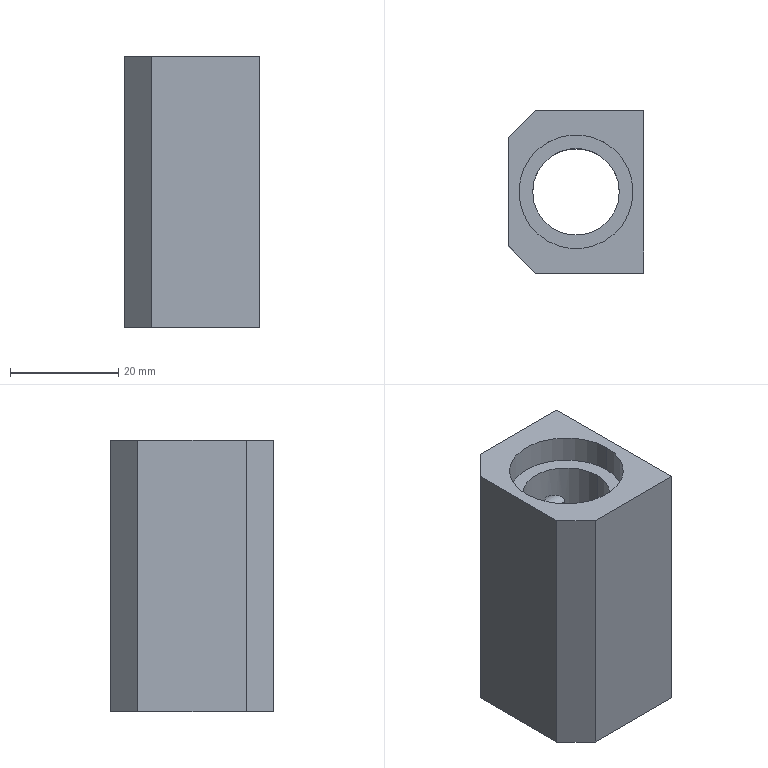Part | STEP file | MT-COMBO-119-S033 | 1 solid | 28 faces | box 25 x 30 x 50 mm | volume 24424 mm3 | cylinder 14 | plane 10 | cone 4 | commonest cylinder face diameters 3.3 x8 21 x4 16 x2
STEP:
#1=CARTESIAN_POINT('',(2.784,-7.5,14.15));
#2=VERTEX_POINT('',#1);
#3=CARTESIAN_POINT('',(2.784,-7.5,10.85));
#4=VERTEX_POINT('',#3);
#5=CARTESIAN_POINT('',(2.784,-7.5,14.15));
#6=CARTESIAN_POINT('',(3.09,-7.386,14.15));
#7=CARTESIAN_POINT('',(3.389,-7.254,14.139));
#8=CARTESIAN_POINT('',(3.967,-6.955,14.065));
#9=CARTESIAN_POINT('',(4.246,-6.787,14.002));
#10=CARTESIAN_POINT('',(4.631,-6.525,13.835));
#11=CARTESIAN_POINT('',(4.753,-6.437,13.767));
#12=CARTESIAN_POINT('',(4.976,-6.266,13.601));
#13=CARTESIAN_POINT('',(5.08,-6.181,13.501));
#14=CARTESIAN_POINT('',(5.256,-6.032,13.266));
#15=CARTESIAN_POINT('',(5.329,-5.967,13.129));
#16=CARTESIAN_POINT('',(5.404,-5.899,12.905));
#17=CARTESIAN_POINT('',(5.424,-5.881,12.828));
#18=CARTESIAN_POINT('',(5.45,-5.856,12.667));
#19=CARTESIAN_POINT('',(5.457,-5.85,12.583));
#20=CARTESIAN_POINT('',(5.457,-5.85,12.337));
#21=CARTESIAN_POINT('',(5.43,-5.875,12.172));
#22=CARTESIAN_POINT('',(5.33,-5.967,11.871));
#23=CARTESIAN_POINT('',(5.257,-6.032,11.734));
#24=CARTESIAN_POINT('',(4.99,-6.257,11.379));
#25=CARTESIAN_POINT('',(4.756,-6.44,11.219));
#26=CARTESIAN_POINT('',(4.246,-6.787,10.998));
#27=CARTESIAN_POINT('',(3.966,-6.955,10.935));
#28=CARTESIAN_POINT('',(3.388,-7.254,10.861));
#29=CARTESIAN_POINT('',(3.09,-7.386,10.85));
#30=CARTESIAN_POINT('',(2.784,-7.5,10.85));
#31=B_SPLINE_CURVE_WITH_KNOTS('',3,(#5,#6,#7,#8,#9,#10,#11,#12,#13,#14,#15,#16,#17,#18,#19,#20,#21,#22,#23,#24,#25,#26,#27,#28,#29,#30),.UNSPECIFIED.,.F.,.F.,(4,2,2,2,2,2,2,2,2,2,2,2,4),(0.0004038,0.001382,0.002361,0.00285,0.003339,0.003829,0.004073,0.004318,0.004807,0.005296,0.006275,0.007253,0.008232),.UNSPECIFIED.);
#32=EDGE_CURVE('',#2,#4,#31,.T.);
#33=ORIENTED_EDGE('',*,*,#32,.T.);
#34=CARTESIAN_POINT('',(12.5,-7.5,10.85));
#35=VERTEX_POINT('',#34);
#36=CARTESIAN_POINT('',(12.5,-7.5,10.85));
#37=DIRECTION('',(1.,0.,0.));
#38=VECTOR('',#37,1000.);
#39=LINE('',#36,#38);
#40=EDGE_CURVE('',#4,#35,#39,.T.);
#41=ORIENTED_EDGE('',*,*,#40,.T.);
#42=CARTESIAN_POINT('',(12.5,-7.5,14.15));
#43=VERTEX_POINT('',#42);
#44=CARTESIAN_POINT('',(12.5,-7.5,12.5));
#45=DIRECTION('',(-1.,0.,0.));
#46=DIRECTION('',(0.,0.,1.));
#47=AXIS2_PLACEMENT_3D('',#44,#45,#46);
#48=CIRCLE('',#47,1.65);
#49=EDGE_CURVE('',#43,#35,#48,.T.);
#50=ORIENTED_EDGE('',*,*,#49,.F.);
#51=CARTESIAN_POINT('',(12.5,-7.5,14.15));
#52=DIRECTION('',(1.,0.,0.));
#53=VECTOR('',#52,1000.);
#54=LINE('',#51,#53);
#55=EDGE_CURVE('',#2,#43,#54,.T.);
#56=ORIENTED_EDGE('',*,*,#55,.F.);
#57=EDGE_LOOP('',(#33,#41,#50,#56));
#58=FACE_OUTER_BOUND('',#57,.T.);
#59=CARTESIAN_POINT('',(12.5,-7.5,12.5));
#60=DIRECTION('',(1.,0.,0.));
#61=DIRECTION('',(0.,0.,1.));
#62=AXIS2_PLACEMENT_3D('',#59,#60,#61);
#63=CYLINDRICAL_SURFACE('',#62,1.65);
#64=ADVANCED_FACE('',(#58),#63,.F.);
#65=CARTESIAN_POINT('',(2.4,7.632,10.855));
#66=VERTEX_POINT('',#65);
#67=CARTESIAN_POINT('',(2.784,7.5,10.85));
#68=VERTEX_POINT('',#67);
#69=CARTESIAN_POINT('',(2.4,7.632,10.855));
#70=CARTESIAN_POINT('',(2.529,7.591,10.852));
#71=CARTESIAN_POINT('',(2.657,7.547,10.85));
#72=CARTESIAN_POINT('',(2.784,7.5,10.85));
#73=B_SPLINE_CURVE_WITH_KNOTS('',3,(#69,#70,#71,#72),.UNSPECIFIED.,.F.,.F.,(4,4),(0.,0.0004038),.UNSPECIFIED.);
#74=EDGE_CURVE('',#66,#68,#73,.T.);
#75=ORIENTED_EDGE('',*,*,#74,.T.);
#76=CARTESIAN_POINT('',(12.5,7.5,10.85));
#77=VERTEX_POINT('',#76);
#78=CARTESIAN_POINT('',(12.5,7.5,10.85));
#79=DIRECTION('',(1.,0.,0.));
#80=VECTOR('',#79,1000.);
#81=LINE('',#78,#80);
#82=EDGE_CURVE('',#68,#77,#81,.T.);
#83=ORIENTED_EDGE('',*,*,#82,.T.);
#84=CARTESIAN_POINT('',(12.5,7.5,14.15));
#85=VERTEX_POINT('',#84);
#86=CARTESIAN_POINT('',(12.5,7.5,12.5));
#87=DIRECTION('',(-1.,0.,0.));
#88=DIRECTION('',(0.,0.,1.));
#89=AXIS2_PLACEMENT_3D('',#86,#87,#88);
#90=CIRCLE('',#89,1.65);
#91=EDGE_CURVE('',#85,#77,#90,.T.);
#92=ORIENTED_EDGE('',*,*,#91,.F.);
#93=CARTESIAN_POINT('',(2.784,7.5,14.15));
#94=VERTEX_POINT('',#93);
#95=CARTESIAN_POINT('',(12.5,7.5,14.15));
#96=DIRECTION('',(1.,0.,0.));
#97=VECTOR('',#96,1000.);
#98=LINE('',#95,#97);
#99=EDGE_CURVE('',#94,#85,#98,.T.);
#100=ORIENTED_EDGE('',*,*,#99,.F.);
#101=CARTESIAN_POINT('',(2.4,7.632,14.145));
#102=VERTEX_POINT('',#101);
#103=CARTESIAN_POINT('',(2.784,7.5,14.15));
#104=CARTESIAN_POINT('',(2.657,7.547,14.15));
#105=CARTESIAN_POINT('',(2.529,7.591,14.148));
#106=CARTESIAN_POINT('',(2.4,7.632,14.145));
#107=B_SPLINE_CURVE_WITH_KNOTS('',3,(#103,#104,#105,#106),.UNSPECIFIED.,.F.,.F.,(4,4),(0.008232,0.008636),.UNSPECIFIED.);
#108=EDGE_CURVE('',#94,#102,#107,.T.);
#109=ORIENTED_EDGE('',*,*,#108,.T.);
#110=CARTESIAN_POINT('',(2.4,7.5,12.5));
#111=DIRECTION('',(-1.,0.,0.));
#112=DIRECTION('',(0.,0.,1.));
#113=AXIS2_PLACEMENT_3D('',#110,#111,#112);
#114=CIRCLE('',#113,1.65);
#115=EDGE_CURVE('',#102,#66,#114,.T.);
#116=ORIENTED_EDGE('',*,*,#115,.T.);
#117=EDGE_LOOP('',(#75,#83,#92,#100,#109,#116));
#118=FACE_OUTER_BOUND('',#117,.T.);
#119=CARTESIAN_POINT('',(12.5,7.5,12.5));
#120=DIRECTION('',(1.,0.,0.));
#121=DIRECTION('',(0.,0.,1.));
#122=AXIS2_PLACEMENT_3D('',#119,#120,#121);
#123=CYLINDRICAL_SURFACE('',#122,1.65);
#124=ADVANCED_FACE('',(#118),#123,.F.);
#125=CARTESIAN_POINT('',(2.4,7.632,-14.145));
#126=VERTEX_POINT('',#125);
#127=CARTESIAN_POINT('',(2.784,7.5,-14.15));
#128=VERTEX_POINT('',#127);
#129=CARTESIAN_POINT('',(2.4,7.632,-14.145));
#130=CARTESIAN_POINT('',(2.529,7.591,-14.148));
#131=CARTESIAN_POINT('',(2.657,7.547,-14.15));
#132=CARTESIAN_POINT('',(2.784,7.5,-14.15));
#133=B_SPLINE_CURVE_WITH_KNOTS('',3,(#129,#130,#131,#132),.UNSPECIFIED.,.F.,.F.,(4,4),(0.,0.0004038),.UNSPECIFIED.);
#134=EDGE_CURVE('',#126,#128,#133,.T.);
#135=ORIENTED_EDGE('',*,*,#134,.T.);
#136=CARTESIAN_POINT('',(12.5,7.5,-14.15));
#137=VERTEX_POINT('',#136);
#138=CARTESIAN_POINT('',(12.5,7.5,-14.15));
#139=DIRECTION('',(1.,0.,0.));
#140=VECTOR('',#139,1000.);
#141=LINE('',#138,#140);
#142=EDGE_CURVE('',#128,#137,#141,.T.);
#143=ORIENTED_EDGE('',*,*,#142,.T.);
#144=CARTESIAN_POINT('',(12.5,7.5,-10.85));
#145=VERTEX_POINT('',#144);
#146=CARTESIAN_POINT('',(12.5,7.5,-12.5));
#147=DIRECTION('',(-1.,0.,0.));
#148=DIRECTION('',(0.,0.,1.));
#149=AXIS2_PLACEMENT_3D('',#146,#147,#148);
#150=CIRCLE('',#149,1.65);
#151=EDGE_CURVE('',#145,#137,#150,.T.);
#152=ORIENTED_EDGE('',*,*,#151,.F.);
#153=CARTESIAN_POINT('',(2.784,7.5,-10.85));
#154=VERTEX_POINT('',#153);
#155=CARTESIAN_POINT('',(12.5,7.5,-10.85));
#156=DIRECTION('',(1.,0.,0.));
#157=VECTOR('',#156,1000.);
#158=LINE('',#155,#157);
#159=EDGE_CURVE('',#154,#145,#158,.T.);
#160=ORIENTED_EDGE('',*,*,#159,.F.);
#161=CARTESIAN_POINT('',(2.4,7.632,-10.855));
#162=VERTEX_POINT('',#161);
#163=CARTESIAN_POINT('',(2.784,7.5,-10.85));
#164=CARTESIAN_POINT('',(2.657,7.547,-10.85));
#165=CARTESIAN_POINT('',(2.529,7.591,-10.852));
#166=CARTESIAN_POINT('',(2.4,7.632,-10.855));
#167=B_SPLINE_CURVE_WITH_KNOTS('',3,(#163,#164,#165,#166),.UNSPECIFIED.,.F.,.F.,(4,4),(0.008232,0.008636),.UNSPECIFIED.);
#168=EDGE_CURVE('',#154,#162,#167,.T.);
#169=ORIENTED_EDGE('',*,*,#168,.T.);
#170=CARTESIAN_POINT('',(2.4,7.5,-12.5));
#171=DIRECTION('',(-1.,0.,0.));
#172=DIRECTION('',(0.,0.,1.));
#173=AXIS2_PLACEMENT_3D('',#170,#171,#172);
#174=CIRCLE('',#173,1.65);
#175=EDGE_CURVE('',#162,#126,#174,.T.);
#176=ORIENTED_EDGE('',*,*,#175,.T.);
#177=EDGE_LOOP('',(#135,#143,#152,#160,#169,#176));
#178=FACE_OUTER_BOUND('',#177,.T.);
#179=CARTESIAN_POINT('',(12.5,7.5,-12.5));
#180=DIRECTION('',(1.,0.,0.));
#181=DIRECTION('',(0.,0.,1.));
#182=AXIS2_PLACEMENT_3D('',#179,#180,#181);
#183=CYLINDRICAL_SURFACE('',#182,1.65);
#184=ADVANCED_FACE('',(#178),#183,.F.);
#185=CARTESIAN_POINT('',(2.784,-7.5,-10.85));
#186=VERTEX_POINT('',#185);
#187=CARTESIAN_POINT('',(2.784,-7.5,-14.15));
#188=VERTEX_POINT('',#187);
#189=CARTESIAN_POINT('',(2.784,-7.5,-10.85));
#190=CARTESIAN_POINT('',(3.09,-7.386,-10.85));
#191=CARTESIAN_POINT('',(3.389,-7.254,-10.861));
#192=CARTESIAN_POINT('',(3.967,-6.955,-10.935));
#193=CARTESIAN_POINT('',(4.246,-6.787,-10.998));
#194=CARTESIAN_POINT('',(4.631,-6.525,-11.165));
#195=CARTESIAN_POINT('',(4.753,-6.437,-11.233));
#196=CARTESIAN_POINT('',(4.976,-6.266,-11.399));
#197=CARTESIAN_POINT('',(5.08,-6.181,-11.499));
#198=CARTESIAN_POINT('',(5.256,-6.032,-11.734));
#199=CARTESIAN_POINT('',(5.329,-5.967,-11.871));
#200=CARTESIAN_POINT('',(5.404,-5.899,-12.095));
#201=CARTESIAN_POINT('',(5.424,-5.881,-12.172));
#202=CARTESIAN_POINT('',(5.45,-5.856,-12.333));
#203=CARTESIAN_POINT('',(5.457,-5.85,-12.417));
#204=CARTESIAN_POINT('',(5.457,-5.85,-12.663));
#205=CARTESIAN_POINT('',(5.43,-5.875,-12.828));
#206=CARTESIAN_POINT('',(5.33,-5.967,-13.129));
#207=CARTESIAN_POINT('',(5.257,-6.032,-13.266));
#208=CARTESIAN_POINT('',(4.99,-6.257,-13.621));
#209=CARTESIAN_POINT('',(4.756,-6.44,-13.781));
#210=CARTESIAN_POINT('',(4.246,-6.787,-14.002));
#211=CARTESIAN_POINT('',(3.966,-6.955,-14.065));
#212=CARTESIAN_POINT('',(3.388,-7.254,-14.139));
#213=CARTESIAN_POINT('',(3.09,-7.386,-14.15));
#214=CARTESIAN_POINT('',(2.784,-7.5,-14.15));
#215=B_SPLINE_CURVE_WITH_KNOTS('',3,(#189,#190,#191,#192,#193,#194,#195,#196,#197,#198,#199,#200,#201,#202,#203,#204,#205,#206,#207,#208,#209,#210,#211,#212,#213,#214),.UNSPECIFIED.,.F.,.F.,(4,2,2,2,2,2,2,2,2,2,2,2,4),(0.0004038,0.001382,0.002361,0.00285,0.003339,0.003829,0.004073,0.004318,0.004807,0.005296,0.006275,0.007253,0.008232),.UNSPECIFIED.);
#216=EDGE_CURVE('',#186,#188,#215,.T.);
#217=ORIENTED_EDGE('',*,*,#216,.T.);
#218=CARTESIAN_POINT('',(12.5,-7.5,-14.15));
#219=VERTEX_POINT('',#218);
#220=CARTESIAN_POINT('',(12.5,-7.5,-14.15));
#221=DIRECTION('',(1.,0.,0.));
#222=VECTOR('',#221,1000.);
#223=LINE('',#220,#222);
#224=EDGE_CURVE('',#188,#219,#223,.T.);
#225=ORIENTED_EDGE('',*,*,#224,.T.);
#226=CARTESIAN_POINT('',(12.5,-7.5,-10.85));
#227=VERTEX_POINT('',#226);
#228=CARTESIAN_POINT('',(12.5,-7.5,-12.5));
#229=DIRECTION('',(-1.,0.,0.));
#230=DIRECTION('',(0.,0.,1.));
#231=AXIS2_PLACEMENT_3D('',#228,#229,#230);
#232=CIRCLE('',#231,1.65);
#233=EDGE_CURVE('',#227,#219,#232,.T.);
#234=ORIENTED_EDGE('',*,*,#233,.F.);
#235=CARTESIAN_POINT('',(12.5,-7.5,-10.85));
#236=DIRECTION('',(1.,0.,0.));
#237=VECTOR('',#236,1000.);
#238=LINE('',#235,#237);
#239=EDGE_CURVE('',#186,#227,#238,.T.);
#240=ORIENTED_EDGE('',*,*,#239,.F.);
#241=EDGE_LOOP('',(#217,#225,#234,#240));
#242=FACE_OUTER_BOUND('',#241,.T.);
#243=CARTESIAN_POINT('',(12.5,-7.5,-12.5));
#244=DIRECTION('',(1.,0.,0.));
#245=DIRECTION('',(0.,0.,1.));
#246=AXIS2_PLACEMENT_3D('',#243,#244,#245);
#247=CYLINDRICAL_SURFACE('',#246,1.65);
#248=ADVANCED_FACE('',(#242),#247,.F.);
#249=CARTESIAN_POINT('',(-10.5,0.,-20.));
#250=VERTEX_POINT('',#249);
#251=CARTESIAN_POINT('',(10.5,0.,-20.));
#252=VERTEX_POINT('',#251);
#253=CARTESIAN_POINT('',(0.,0.,-20.));
#254=DIRECTION('',(0.,0.,-1.));
#255=DIRECTION('',(-1.,0.,0.));
#256=AXIS2_PLACEMENT_3D('',#253,#254,#255);
#257=CIRCLE('',#256,10.5);
#258=EDGE_CURVE('',#250,#252,#257,.T.);
#259=ORIENTED_EDGE('',*,*,#258,.F.);
#260=CARTESIAN_POINT('',(-10.5,0.,-25.));
#261=VERTEX_POINT('',#260);
#262=CARTESIAN_POINT('',(-10.5,0.,-20.));
#263=DIRECTION('',(0.,0.,-1.));
#264=VECTOR('',#263,1000.);
#265=LINE('',#262,#264);
#266=EDGE_CURVE('',#250,#261,#265,.T.);
#267=ORIENTED_EDGE('',*,*,#266,.T.);
#268=CARTESIAN_POINT('',(10.5,0.,-25.));
#269=VERTEX_POINT('',#268);
#270=CARTESIAN_POINT('',(0.,0.,-25.));
#271=DIRECTION('',(0.,0.,-1.));
#272=DIRECTION('',(-1.,0.,0.));
#273=AXIS2_PLACEMENT_3D('',#270,#271,#272);
#274=CIRCLE('',#273,10.5);
#275=EDGE_CURVE('',#261,#269,#274,.T.);
#276=ORIENTED_EDGE('',*,*,#275,.T.);
#277=CARTESIAN_POINT('',(10.5,0.,-20.));
#278=DIRECTION('',(0.,0.,-1.));
#279=VECTOR('',#278,1000.);
#280=LINE('',#277,#279);
#281=EDGE_CURVE('',#252,#269,#280,.T.);
#282=ORIENTED_EDGE('',*,*,#281,.F.);
#283=EDGE_LOOP('',(#259,#267,#276,#282));
#284=FACE_OUTER_BOUND('',#283,.T.);
#285=CARTESIAN_POINT('',(0.,0.,-20.));
#286=DIRECTION('',(0.,0.,-1.));
#287=DIRECTION('',(1.,0.,0.));
#288=AXIS2_PLACEMENT_3D('',#285,#286,#287);
#289=CYLINDRICAL_SURFACE('',#288,10.5);
#290=ADVANCED_FACE('',(#284),#289,.F.);
#291=CARTESIAN_POINT('',(-10.5,0.,20.));
#292=VERTEX_POINT('',#291);
#293=CARTESIAN_POINT('',(10.5,0.,20.));
#294=VERTEX_POINT('',#293);
#295=CARTESIAN_POINT('',(0.,0.,20.));
#296=DIRECTION('',(0.,0.,-1.));
#297=DIRECTION('',(-1.,0.,0.));
#298=AXIS2_PLACEMENT_3D('',#295,#296,#297);
#299=CIRCLE('',#298,10.5);
#300=EDGE_CURVE('',#292,#294,#299,.T.);
#301=ORIENTED_EDGE('',*,*,#300,.T.);
#302=CARTESIAN_POINT('',(10.5,0.,25.));
#303=VERTEX_POINT('',#302);
#304=CARTESIAN_POINT('',(10.5,0.,20.));
#305=DIRECTION('',(0.,0.,1.));
#306=VECTOR('',#305,1000.);
#307=LINE('',#304,#306);
#308=EDGE_CURVE('',#294,#303,#307,.T.);
#309=ORIENTED_EDGE('',*,*,#308,.T.);
#310=CARTESIAN_POINT('',(-10.5,0.,25.));
#311=VERTEX_POINT('',#310);
#312=CARTESIAN_POINT('',(0.,0.,25.));
#313=DIRECTION('',(0.,0.,-1.));
#314=DIRECTION('',(-1.,0.,0.));
#315=AXIS2_PLACEMENT_3D('',#312,#313,#314);
#316=CIRCLE('',#315,10.5);
#317=EDGE_CURVE('',#311,#303,#316,.T.);
#318=ORIENTED_EDGE('',*,*,#317,.F.);
#319=CARTESIAN_POINT('',(-10.5,0.,20.));
#320=DIRECTION('',(0.,0.,1.));
#321=VECTOR('',#320,1000.);
#322=LINE('',#319,#321);
#323=EDGE_CURVE('',#292,#311,#322,.T.);
#324=ORIENTED_EDGE('',*,*,#323,.F.);
#325=EDGE_LOOP('',(#301,#309,#318,#324));
#326=FACE_OUTER_BOUND('',#325,.T.);
#327=CARTESIAN_POINT('',(0.,0.,20.));
#328=DIRECTION('',(0.,0.,1.));
#329=DIRECTION('',(-1.,0.,0.));
#330=AXIS2_PLACEMENT_3D('',#327,#328,#329);
#331=CYLINDRICAL_SURFACE('',#330,10.5);
#332=ADVANCED_FACE('',(#326),#331,.F.);
#333=CARTESIAN_POINT('',(2.4,7.632,-10.855));
#334=CARTESIAN_POINT('',(2.244,7.68,-11.119));
#335=CARTESIAN_POINT('',(2.089,7.724,-11.384));
#336=CARTESIAN_POINT('',(1.867,7.78,-11.789));
#337=CARTESIAN_POINT('',(1.794,7.797,-11.924));
#338=CARTESIAN_POINT('',(1.698,7.818,-12.135));
#339=CARTESIAN_POINT('',(1.668,7.824,-12.207));
#340=CARTESIAN_POINT('',(1.624,7.834,-12.355));
#341=CARTESIAN_POINT('',(1.61,7.836,-12.432));
#342=CARTESIAN_POINT('',(1.612,7.836,-12.586));
#343=CARTESIAN_POINT('',(1.628,7.833,-12.663));
#344=CARTESIAN_POINT('',(1.675,7.823,-12.81));
#345=CARTESIAN_POINT('',(1.704,7.816,-12.88));
#346=CARTESIAN_POINT('',(1.8,7.795,-13.087));
#347=CARTESIAN_POINT('',(1.872,7.778,-13.222));
#348=CARTESIAN_POINT('',(2.093,7.723,-13.622));
#349=CARTESIAN_POINT('',(2.246,7.68,-13.884));
#350=CARTESIAN_POINT('',(2.4,7.632,-14.145));
#351=B_SPLINE_CURVE_WITH_KNOTS('',3,(#333,#334,#335,#336,#337,#338,#339,#340,#341,#342,#343,#344,#345,#346,#347,#348,#349,#350),.UNSPECIFIED.,.F.,.F.,(4,2,2,2,2,2,2,2,4),(0.0001976,0.001128,0.001593,0.001825,0.002058,0.00229,0.002523,0.002988,0.003918),.UNSPECIFIED.);
#352=EDGE_CURVE('',#162,#126,#351,.T.);
#353=ORIENTED_EDGE('',*,*,#352,.F.);
#354=ORIENTED_EDGE('',*,*,#168,.F.);
#355=CARTESIAN_POINT('',(2.784,7.5,-14.15));
#356=CARTESIAN_POINT('',(3.09,7.386,-14.15));
#357=CARTESIAN_POINT('',(3.389,7.254,-14.139));
#358=CARTESIAN_POINT('',(3.967,6.955,-14.065));
#359=CARTESIAN_POINT('',(4.246,6.787,-14.002));
#360=CARTESIAN_POINT('',(4.631,6.525,-13.835));
#361=CARTESIAN_POINT('',(4.753,6.437,-13.767));
#362=CARTESIAN_POINT('',(4.976,6.266,-13.601));
#363=CARTESIAN_POINT('',(5.08,6.181,-13.501));
#364=CARTESIAN_POINT('',(5.256,6.032,-13.266));
#365=CARTESIAN_POINT('',(5.329,5.967,-13.129));
#366=CARTESIAN_POINT('',(5.404,5.899,-12.905));
#367=CARTESIAN_POINT('',(5.424,5.881,-12.828));
#368=CARTESIAN_POINT('',(5.45,5.856,-12.667));
#369=CARTESIAN_POINT('',(5.457,5.85,-12.583));
#370=CARTESIAN_POINT('',(5.457,5.85,-12.337));
#371=CARTESIAN_POINT('',(5.43,5.875,-12.172));
#372=CARTESIAN_POINT('',(5.33,5.967,-11.871));
#373=CARTESIAN_POINT('',(5.257,6.032,-11.734));
#374=CARTESIAN_POINT('',(4.99,6.257,-11.379));
#375=CARTESIAN_POINT('',(4.756,6.44,-11.219));
#376=CARTESIAN_POINT('',(4.246,6.787,-10.998));
#377=CARTESIAN_POINT('',(3.966,6.955,-10.935));
#378=CARTESIAN_POINT('',(3.388,7.254,-10.861));
#379=CARTESIAN_POINT('',(3.09,7.386,-10.85));
#380=CARTESIAN_POINT('',(2.784,7.5,-10.85));
#381=B_SPLINE_CURVE_WITH_KNOTS('',3,(#355,#356,#357,#358,#359,#360,#361,#362,#363,#364,#365,#366,#367,#368,#369,#370,#371,#372,#373,#374,#375,#376,#377,#378,#379,#380),.UNSPECIFIED.,.F.,.F.,(4,2,2,2,2,2,2,2,2,2,2,2,4),(0.0004038,0.001382,0.002361,0.00285,0.003339,0.003829,0.004073,0.004318,0.004807,0.005296,0.006275,0.007253,0.008232),.UNSPECIFIED.);
#382=EDGE_CURVE('',#128,#154,#381,.T.);
#383=ORIENTED_EDGE('',*,*,#382,.F.);
#384=ORIENTED_EDGE('',*,*,#134,.F.);
#385=EDGE_LOOP('',(#353,#354,#383,#384));
#386=FACE_BOUND('',#385,.T.);
#387=CARTESIAN_POINT('',(2.4,7.632,14.145));
#388=CARTESIAN_POINT('',(2.244,7.68,13.881));
#389=CARTESIAN_POINT('',(2.089,7.724,13.616));
#390=CARTESIAN_POINT('',(1.867,7.78,13.211));
#391=CARTESIAN_POINT('',(1.794,7.797,13.076));
#392=CARTESIAN_POINT('',(1.698,7.818,12.865));
#393=CARTESIAN_POINT('',(1.668,7.824,12.793));
#394=CARTESIAN_POINT('',(1.624,7.834,12.645));
#395=CARTESIAN_POINT('',(1.61,7.836,12.568));
#396=CARTESIAN_POINT('',(1.612,7.836,12.414));
#397=CARTESIAN_POINT('',(1.628,7.833,12.337));
#398=CARTESIAN_POINT('',(1.675,7.823,12.19));
#399=CARTESIAN_POINT('',(1.704,7.816,12.12));
#400=CARTESIAN_POINT('',(1.8,7.795,11.913));
#401=CARTESIAN_POINT('',(1.872,7.778,11.778));
#402=CARTESIAN_POINT('',(2.093,7.723,11.378));
#403=CARTESIAN_POINT('',(2.246,7.68,11.116));
#404=CARTESIAN_POINT('',(2.4,7.632,10.855));
#405=B_SPLINE_CURVE_WITH_KNOTS('',3,(#387,#388,#389,#390,#391,#392,#393,#394,#395,#396,#397,#398,#399,#400,#401,#402,#403,#404),.UNSPECIFIED.,.F.,.F.,(4,2,2,2,2,2,2,2,4),(0.0001976,0.001128,0.001593,0.001825,0.002058,0.00229,0.002523,0.002988,0.003918),.UNSPECIFIED.);
#406=EDGE_CURVE('',#102,#66,#405,.T.);
#407=ORIENTED_EDGE('',*,*,#406,.F.);
#408=ORIENTED_EDGE('',*,*,#108,.F.);
#409=CARTESIAN_POINT('',(2.784,7.5,10.85));
#410=CARTESIAN_POINT('',(3.09,7.386,10.85));
#411=CARTESIAN_POINT('',(3.389,7.254,10.861));
#412=CARTESIAN_POINT('',(3.967,6.955,10.935));
#413=CARTESIAN_POINT('',(4.246,6.787,10.998));
#414=CARTESIAN_POINT('',(4.631,6.525,11.165));
#415=CARTESIAN_POINT('',(4.753,6.437,11.233));
#416=CARTESIAN_POINT('',(4.976,6.266,11.399));
#417=CARTESIAN_POINT('',(5.08,6.181,11.499));
#418=CARTESIAN_POINT('',(5.256,6.032,11.734));
#419=CARTESIAN_POINT('',(5.329,5.967,11.871));
#420=CARTESIAN_POINT('',(5.404,5.899,12.095));
#421=CARTESIAN_POINT('',(5.424,5.881,12.172));
#422=CARTESIAN_POINT('',(5.45,5.856,12.333));
#423=CARTESIAN_POINT('',(5.457,5.85,12.417));
#424=CARTESIAN_POINT('',(5.457,5.85,12.663));
#425=CARTESIAN_POINT('',(5.43,5.875,12.828));
#426=CARTESIAN_POINT('',(5.33,5.967,13.129));
#427=CARTESIAN_POINT('',(5.257,6.032,13.266));
#428=CARTESIAN_POINT('',(4.99,6.257,13.621));
#429=CARTESIAN_POINT('',(4.756,6.44,13.781));
#430=CARTESIAN_POINT('',(4.246,6.787,14.002));
#431=CARTESIAN_POINT('',(3.966,6.955,14.065));
#432=CARTESIAN_POINT('',(3.388,7.254,14.139));
#433=CARTESIAN_POINT('',(3.09,7.386,14.15));
#434=CARTESIAN_POINT('',(2.784,7.5,14.15));
#435=B_SPLINE_CURVE_WITH_KNOTS('',3,(#409,#410,#411,#412,#413,#414,#415,#416,#417,#418,#419,#420,#421,#422,#423,#424,#425,#426,#427,#428,#429,#430,#431,#432,#433,#434),.UNSPECIFIED.,.F.,.F.,(4,2,2,2,2,2,2,2,2,2,2,2,4),(0.0004038,0.001382,0.002361,0.00285,0.003339,0.003829,0.004073,0.004318,0.004807,0.005296,0.006275,0.007253,0.008232),.UNSPECIFIED.);
#436=EDGE_CURVE('',#68,#94,#435,.T.);
#437=ORIENTED_EDGE('',*,*,#436,.F.);
#438=ORIENTED_EDGE('',*,*,#74,.F.);
#439=EDGE_LOOP('',(#407,#408,#437,#438));
#440=FACE_BOUND('',#439,.T.);
#441=CARTESIAN_POINT('',(8.,0.,20.));
#442=VERTEX_POINT('',#441);
#443=CARTESIAN_POINT('',(-8.,0.,20.));
#444=VERTEX_POINT('',#443);
#445=CARTESIAN_POINT('',(0.,0.,20.));
#446=DIRECTION('',(0.,0.,1.));
#447=DIRECTION('',(-1.,0.,0.));
#448=AXIS2_PLACEMENT_3D('',#445,#446,#447);
#449=CIRCLE('',#448,8.);
#450=EDGE_CURVE('',#442,#444,#449,.T.);
#451=ORIENTED_EDGE('',*,*,#450,.T.);
#452=CARTESIAN_POINT('',(-8.,0.,-20.));
#453=VERTEX_POINT('',#452);
#454=CARTESIAN_POINT('',(-8.,0.,25.));
#455=DIRECTION('',(0.,0.,-1.));
#456=VECTOR('',#455,1000.);
#457=LINE('',#454,#456);
#458=EDGE_CURVE('',#444,#453,#457,.T.);
#459=ORIENTED_EDGE('',*,*,#458,.T.);
#460=CARTESIAN_POINT('',(8.,0.,-20.));
#461=VERTEX_POINT('',#460);
#462=CARTESIAN_POINT('',(0.,0.,-20.));
#463=DIRECTION('',(0.,0.,-1.));
#464=DIRECTION('',(1.,0.,0.));
#465=AXIS2_PLACEMENT_3D('',#462,#463,#464);
#466=CIRCLE('',#465,8.);
#467=EDGE_CURVE('',#453,#461,#466,.T.);
#468=ORIENTED_EDGE('',*,*,#467,.T.);
#469=CARTESIAN_POINT('',(8.,0.,25.));
#470=DIRECTION('',(0.,0.,-1.));
#471=VECTOR('',#470,1000.);
#472=LINE('',#469,#471);
#473=EDGE_CURVE('',#442,#461,#472,.T.);
#474=ORIENTED_EDGE('',*,*,#473,.F.);
#475=EDGE_LOOP('',(#451,#459,#468,#474));
#476=FACE_OUTER_BOUND('',#475,.T.);
#477=CARTESIAN_POINT('',(0.,0.,25.));
#478=DIRECTION('',(0.,0.,-1.));
#479=DIRECTION('',(1.,0.,0.));
#480=AXIS2_PLACEMENT_3D('',#477,#478,#479);
#481=CYLINDRICAL_SURFACE('',#480,8.);
#482=ADVANCED_FACE('',(#386,#440,#476),#481,.F.);
#483=ORIENTED_EDGE('',*,*,#458,.F.);
#484=CARTESIAN_POINT('',(0.,0.,20.));
#485=DIRECTION('',(0.,0.,1.));
#486=DIRECTION('',(-1.,0.,0.));
#487=AXIS2_PLACEMENT_3D('',#484,#485,#486);
#488=CIRCLE('',#487,8.);
#489=EDGE_CURVE('',#444,#442,#488,.T.);
#490=ORIENTED_EDGE('',*,*,#489,.T.);
#491=ORIENTED_EDGE('',*,*,#473,.T.);
#492=CARTESIAN_POINT('',(0.,0.,-20.));
#493=DIRECTION('',(0.,0.,-1.));
#494=DIRECTION('',(1.,0.,0.));
#495=AXIS2_PLACEMENT_3D('',#492,#493,#494);
#496=CIRCLE('',#495,8.);
#497=EDGE_CURVE('',#461,#453,#496,.T.);
#498=ORIENTED_EDGE('',*,*,#497,.T.);
#499=EDGE_LOOP('',(#483,#490,#491,#498));
#500=FACE_OUTER_BOUND('',#499,.T.);
#501=CARTESIAN_POINT('',(2.4,-7.632,10.855));
#502=VERTEX_POINT('',#501);
#503=CARTESIAN_POINT('',(2.4,-7.632,14.145));
#504=VERTEX_POINT('',#503);
#505=CARTESIAN_POINT('',(2.4,-7.632,10.855));
#506=CARTESIAN_POINT('',(2.244,-7.68,11.119));
#507=CARTESIAN_POINT('',(2.089,-7.724,11.384));
#508=CARTESIAN_POINT('',(1.867,-7.78,11.789));
#509=CARTESIAN_POINT('',(1.794,-7.797,11.924));
#510=CARTESIAN_POINT('',(1.698,-7.818,12.135));
#511=CARTESIAN_POINT('',(1.668,-7.824,12.207));
#512=CARTESIAN_POINT('',(1.624,-7.834,12.355));
#513=CARTESIAN_POINT('',(1.61,-7.836,12.432));
#514=CARTESIAN_POINT('',(1.612,-7.836,12.586));
#515=CARTESIAN_POINT('',(1.628,-7.833,12.663));
#516=CARTESIAN_POINT('',(1.675,-7.823,12.81));
#517=CARTESIAN_POINT('',(1.704,-7.816,12.88));
#518=CARTESIAN_POINT('',(1.8,-7.795,13.087));
#519=CARTESIAN_POINT('',(1.872,-7.778,13.222));
#520=CARTESIAN_POINT('',(2.093,-7.723,13.622));
#521=CARTESIAN_POINT('',(2.246,-7.68,13.884));
#522=CARTESIAN_POINT('',(2.4,-7.632,14.145));
#523=B_SPLINE_CURVE_WITH_KNOTS('',3,(#505,#506,#507,#508,#509,#510,#511,#512,#513,#514,#515,#516,#517,#518,#519,#520,#521,#522),.UNSPECIFIED.,.F.,.F.,(4,2,2,2,2,2,2,2,4),(0.0001976,0.001128,0.001593,0.001825,0.002058,0.00229,0.002523,0.002988,0.003918),.UNSPECIFIED.);
#524=EDGE_CURVE('',#502,#504,#523,.T.);
#525=ORIENTED_EDGE('',*,*,#524,.F.);
#526=CARTESIAN_POINT('',(2.784,-7.5,10.85));
#527=CARTESIAN_POINT('',(2.657,-7.547,10.85));
#528=CARTESIAN_POINT('',(2.529,-7.591,10.852));
#529=CARTESIAN_POINT('',(2.4,-7.632,10.855));
#530=B_SPLINE_CURVE_WITH_KNOTS('',3,(#526,#527,#528,#529),.UNSPECIFIED.,.F.,.F.,(4,4),(0.008232,0.008636),.UNSPECIFIED.);
#531=EDGE_CURVE('',#4,#502,#530,.T.);
#532=ORIENTED_EDGE('',*,*,#531,.F.);
#533=ORIENTED_EDGE('',*,*,#32,.F.);
#534=CARTESIAN_POINT('',(2.4,-7.632,14.145));
#535=CARTESIAN_POINT('',(2.529,-7.591,14.148));
#536=CARTESIAN_POINT('',(2.657,-7.547,14.15));
#537=CARTESIAN_POINT('',(2.784,-7.5,14.15));
#538=B_SPLINE_CURVE_WITH_KNOTS('',3,(#534,#535,#536,#537),.UNSPECIFIED.,.F.,.F.,(4,4),(0.,0.0004038),.UNSPECIFIED.);
#539=EDGE_CURVE('',#504,#2,#538,.T.);
#540=ORIENTED_EDGE('',*,*,#539,.F.);
#541=EDGE_LOOP('',(#525,#532,#533,#540));
#542=FACE_BOUND('',#541,.T.);
#543=CARTESIAN_POINT('',(2.4,-7.632,-14.145));
#544=VERTEX_POINT('',#543);
#545=CARTESIAN_POINT('',(2.4,-7.632,-10.855));
#546=VERTEX_POINT('',#545);
#547=CARTESIAN_POINT('',(2.4,-7.632,-14.145));
#548=CARTESIAN_POINT('',(2.244,-7.68,-13.881));
#549=CARTESIAN_POINT('',(2.089,-7.724,-13.616));
#550=CARTESIAN_POINT('',(1.867,-7.78,-13.211));
#551=CARTESIAN_POINT('',(1.794,-7.797,-13.076));
#552=CARTESIAN_POINT('',(1.698,-7.818,-12.865));
#553=CARTESIAN_POINT('',(1.668,-7.824,-12.793));
#554=CARTESIAN_POINT('',(1.624,-7.834,-12.645));
#555=CARTESIAN_POINT('',(1.61,-7.836,-12.568));
#556=CARTESIAN_POINT('',(1.612,-7.836,-12.414));
#557=CARTESIAN_POINT('',(1.628,-7.833,-12.337));
#558=CARTESIAN_POINT('',(1.675,-7.823,-12.19));
#559=CARTESIAN_POINT('',(1.704,-7.816,-12.12));
#560=CARTESIAN_POINT('',(1.8,-7.795,-11.913));
#561=CARTESIAN_POINT('',(1.872,-7.778,-11.778));
#562=CARTESIAN_POINT('',(2.093,-7.723,-11.378));
#563=CARTESIAN_POINT('',(2.246,-7.68,-11.116));
#564=CARTESIAN_POINT('',(2.4,-7.632,-10.855));
#565=B_SPLINE_CURVE_WITH_KNOTS('',3,(#547,#548,#549,#550,#551,#552,#553,#554,#555,#556,#557,#558,#559,#560,#561,#562,#563,#564),.UNSPECIFIED.,.F.,.F.,(4,2,2,2,2,2,2,2,4),(0.0001976,0.001128,0.001593,0.001825,0.002058,0.00229,0.002523,0.002988,0.003918),.UNSPECIFIED.);
#566=EDGE_CURVE('',#544,#546,#565,.T.);
#567=ORIENTED_EDGE('',*,*,#566,.F.);
#568=CARTESIAN_POINT('',(2.784,-7.5,-14.15));
#569=CARTESIAN_POINT('',(2.657,-7.547,-14.15));
#570=CARTESIAN_POINT('',(2.529,-7.591,-14.148));
#571=CARTESIAN_POINT('',(2.4,-7.632,-14.145));
#572=B_SPLINE_CURVE_WITH_KNOTS('',3,(#568,#569,#570,#571),.UNSPECIFIED.,.F.,.F.,(4,4),(0.008232,0.008636),.UNSPECIFIED.);
#573=EDGE_CURVE('',#188,#544,#572,.T.);
#574=ORIENTED_EDGE('',*,*,#573,.F.);
#575=ORIENTED_EDGE('',*,*,#216,.F.);
#576=CARTESIAN_POINT('',(2.4,-7.632,-10.855));
#577=CARTESIAN_POINT('',(2.529,-7.591,-10.852));
#578=CARTESIAN_POINT('',(2.657,-7.547,-10.85));
#579=CARTESIAN_POINT('',(2.784,-7.5,-10.85));
#580=B_SPLINE_CURVE_WITH_KNOTS('',3,(#576,#577,#578,#579),.UNSPECIFIED.,.F.,.F.,(4,4),(0.,0.0004038),.UNSPECIFIED.);
#581=EDGE_CURVE('',#546,#186,#580,.T.);
#582=ORIENTED_EDGE('',*,*,#581,.F.);
#583=EDGE_LOOP('',(#567,#574,#575,#582));
#584=FACE_BOUND('',#583,.T.);
#585=CARTESIAN_POINT('',(0.,0.,25.));
#586=DIRECTION('',(0.,0.,-1.));
#587=DIRECTION('',(1.,0.,0.));
#588=AXIS2_PLACEMENT_3D('',#585,#586,#587);
#589=CYLINDRICAL_SURFACE('',#588,8.);
#590=ADVANCED_FACE('',(#500,#542,#584),#589,.F.);
#591=ORIENTED_EDGE('',*,*,#49,.T.);
#592=CARTESIAN_POINT('',(12.5,-7.5,12.5));
#593=DIRECTION('',(-1.,0.,0.));
#594=DIRECTION('',(0.,0.,1.));
#595=AXIS2_PLACEMENT_3D('',#592,#593,#594);
#596=CIRCLE('',#595,1.65);
#597=EDGE_CURVE('',#35,#43,#596,.T.);
#598=ORIENTED_EDGE('',*,*,#597,.T.);
#599=EDGE_LOOP('',(#591,#598));
#600=FACE_BOUND('',#599,.T.);
#601=ORIENTED_EDGE('',*,*,#91,.T.);
#602=CARTESIAN_POINT('',(12.5,7.5,12.5));
#603=DIRECTION('',(-1.,0.,0.));
#604=DIRECTION('',(0.,0.,1.));
#605=AXIS2_PLACEMENT_3D('',#602,#603,#604);
#606=CIRCLE('',#605,1.65);
#607=EDGE_CURVE('',#77,#85,#606,.T.);
#608=ORIENTED_EDGE('',*,*,#607,.T.);
#609=EDGE_LOOP('',(#601,#608));
#610=FACE_BOUND('',#609,.T.);
#611=ORIENTED_EDGE('',*,*,#151,.T.);
#612=CARTESIAN_POINT('',(12.5,7.5,-12.5));
#613=DIRECTION('',(-1.,0.,0.));
#614=DIRECTION('',(0.,0.,1.));
#615=AXIS2_PLACEMENT_3D('',#612,#613,#614);
#616=CIRCLE('',#615,1.65);
#617=EDGE_CURVE('',#137,#145,#616,.T.);
#618=ORIENTED_EDGE('',*,*,#617,.T.);
#619=EDGE_LOOP('',(#611,#618));
#620=FACE_BOUND('',#619,.T.);
#621=ORIENTED_EDGE('',*,*,#233,.T.);
#622=CARTESIAN_POINT('',(12.5,-7.5,-12.5));
#623=DIRECTION('',(-1.,0.,0.));
#624=DIRECTION('',(0.,0.,1.));
#625=AXIS2_PLACEMENT_3D('',#622,#623,#624);
#626=CIRCLE('',#625,1.65);
#627=EDGE_CURVE('',#219,#227,#626,.T.);
#628=ORIENTED_EDGE('',*,*,#627,.T.);
#629=EDGE_LOOP('',(#621,#628));
#630=FACE_BOUND('',#629,.T.);
#631=CARTESIAN_POINT('',(12.5,-15.,25.));
#632=VERTEX_POINT('',#631);
#633=CARTESIAN_POINT('',(12.5,15.,25.));
#634=VERTEX_POINT('',#633);
#635=CARTESIAN_POINT('',(12.5,15.,25.));
#636=DIRECTION('',(0.,1.,0.));
#637=VECTOR('',#636,1000.);
#638=LINE('',#635,#637);
#639=EDGE_CURVE('',#632,#634,#638,.T.);
#640=ORIENTED_EDGE('',*,*,#639,.F.);
#641=CARTESIAN_POINT('',(12.5,-15.,-25.));
#642=VERTEX_POINT('',#641);
#643=CARTESIAN_POINT('',(12.5,-15.,-25.));
#644=DIRECTION('',(0.,0.,1.));
#645=VECTOR('',#644,1000.);
#646=LINE('',#643,#645);
#647=EDGE_CURVE('',#642,#632,#646,.T.);
#648=ORIENTED_EDGE('',*,*,#647,.F.);
#649=CARTESIAN_POINT('',(12.5,15.,-25.));
#650=VERTEX_POINT('',#649);
#651=CARTESIAN_POINT('',(12.5,15.,-25.));
#652=DIRECTION('',(0.,1.,0.));
#653=VECTOR('',#652,1000.);
#654=LINE('',#651,#653);
#655=EDGE_CURVE('',#642,#650,#654,.T.);
#656=ORIENTED_EDGE('',*,*,#655,.T.);
#657=CARTESIAN_POINT('',(12.5,15.,-25.));
#658=DIRECTION('',(0.,0.,1.));
#659=VECTOR('',#658,1000.);
#660=LINE('',#657,#659);
#661=EDGE_CURVE('',#650,#634,#660,.T.);
#662=ORIENTED_EDGE('',*,*,#661,.T.);
#663=EDGE_LOOP('',(#640,#648,#656,#662));
#664=FACE_OUTER_BOUND('',#663,.T.);
#665=CARTESIAN_POINT('',(12.5,15.,-25.));
#666=DIRECTION('',(-1.,0.,0.));
#667=DIRECTION('',(0.,0.,-1.));
#668=AXIS2_PLACEMENT_3D('',#665,#666,#667);
#669=PLANE('',#668);
#670=ADVANCED_FACE('',(#600,#610,#620,#630,#664),#669,.F.);
#671=CARTESIAN_POINT('',(-7.5,15.,25.));
#672=VERTEX_POINT('',#671);
#673=CARTESIAN_POINT('',(12.5,15.,25.));
#674=DIRECTION('',(-1.,0.,0.));
#675=VECTOR('',#674,1000.);
#676=LINE('',#673,#675);
#677=EDGE_CURVE('',#634,#672,#676,.T.);
#678=ORIENTED_EDGE('',*,*,#677,.F.);
#679=ORIENTED_EDGE('',*,*,#661,.F.);
#680=CARTESIAN_POINT('',(-7.5,15.,-25.));
#681=VERTEX_POINT('',#680);
#682=CARTESIAN_POINT('',(12.5,15.,-25.));
#683=DIRECTION('',(-1.,0.,0.));
#684=VECTOR('',#683,1000.);
#685=LINE('',#682,#684);
#686=EDGE_CURVE('',#650,#681,#685,.T.);
#687=ORIENTED_EDGE('',*,*,#686,.T.);
#688=CARTESIAN_POINT('',(-7.5,15.,-25.));
#689=DIRECTION('',(0.,0.,-1.));
#690=VECTOR('',#689,1000.);
#691=LINE('',#688,#690);
#692=EDGE_CURVE('',#672,#681,#691,.T.);
#693=ORIENTED_EDGE('',*,*,#692,.F.);
#694=EDGE_LOOP('',(#678,#679,#687,#693));
#695=FACE_OUTER_BOUND('',#694,.T.);
#696=CARTESIAN_POINT('',(12.5,15.,-25.));
#697=DIRECTION('',(0.,-1.,0.));
#698=DIRECTION('',(0.,0.,1.));
#699=AXIS2_PLACEMENT_3D('',#696,#697,#698);
#700=PLANE('',#699);
#701=ADVANCED_FACE('',(#695),#700,.F.);
#702=CARTESIAN_POINT('',(-12.5,10.,-25.));
#703=VERTEX_POINT('',#702);
#704=CARTESIAN_POINT('',(-12.5,-10.,-25.));
#705=VERTEX_POINT('',#704);
#706=CARTESIAN_POINT('',(-12.5,15.,-25.));
#707=DIRECTION('',(0.,-1.,0.));
#708=VECTOR('',#707,1000.);
#709=LINE('',#706,#708);
#710=EDGE_CURVE('',#703,#705,#709,.T.);
#711=ORIENTED_EDGE('',*,*,#710,.T.);
#712=CARTESIAN_POINT('',(-12.5,-10.,25.));
#713=VERTEX_POINT('',#712);
#714=CARTESIAN_POINT('',(-12.5,-10.,-25.));
#715=DIRECTION('',(0.,0.,-1.));
#716=VECTOR('',#715,1000.);
#717=LINE('',#714,#716);
#718=EDGE_CURVE('',#713,#705,#717,.T.);
#719=ORIENTED_EDGE('',*,*,#718,.F.);
#720=CARTESIAN_POINT('',(-12.5,10.,25.));
#721=VERTEX_POINT('',#720);
#722=CARTESIAN_POINT('',(-12.5,15.,25.));
#723=DIRECTION('',(0.,-1.,0.));
#724=VECTOR('',#723,1000.);
#725=LINE('',#722,#724);
#726=EDGE_CURVE('',#721,#713,#725,.T.);
#727=ORIENTED_EDGE('',*,*,#726,.F.);
#728=CARTESIAN_POINT('',(-12.5,10.,-25.));
#729=DIRECTION('',(0.,0.,1.));
#730=VECTOR('',#729,1000.);
#731=LINE('',#728,#730);
#732=EDGE_CURVE('',#703,#721,#731,.T.);
#733=ORIENTED_EDGE('',*,*,#732,.F.);
#734=EDGE_LOOP('',(#711,#719,#727,#733));
#735=FACE_OUTER_BOUND('',#734,.T.);
#736=CARTESIAN_POINT('',(-12.5,15.,-25.));
#737=DIRECTION('',(1.,0.,0.));
#738=DIRECTION('',(0.,1.,0.));
#739=AXIS2_PLACEMENT_3D('',#736,#737,#738);
#740=PLANE('',#739);
#741=ADVANCED_FACE('',(#735),#740,.F.);
#742=CARTESIAN_POINT('',(-7.5,-15.,-25.));
#743=VERTEX_POINT('',#742);
#744=CARTESIAN_POINT('',(12.5,-15.,-25.));
#745=DIRECTION('',(1.,0.,0.));
#746=VECTOR('',#745,1000.);
#747=LINE('',#744,#746);
#748=EDGE_CURVE('',#743,#642,#747,.T.);
#749=ORIENTED_EDGE('',*,*,#748,.T.);
#750=ORIENTED_EDGE('',*,*,#647,.T.);
#751=CARTESIAN_POINT('',(-7.5,-15.,25.));
#752=VERTEX_POINT('',#751);
#753=CARTESIAN_POINT('',(12.5,-15.,25.));
#754=DIRECTION('',(1.,0.,0.));
#755=VECTOR('',#754,1000.);
#756=LINE('',#753,#755);
#757=EDGE_CURVE('',#752,#632,#756,.T.);
#758=ORIENTED_EDGE('',*,*,#757,.F.);
#759=CARTESIAN_POINT('',(-7.5,-15.,-25.));
#760=DIRECTION('',(0.,0.,1.));
#761=VECTOR('',#760,1000.);
#762=LINE('',#759,#761);
#763=EDGE_CURVE('',#743,#752,#762,.T.);
#764=ORIENTED_EDGE('',*,*,#763,.F.);
#765=EDGE_LOOP('',(#749,#750,#758,#764));
#766=FACE_OUTER_BOUND('',#765,.T.);
#767=CARTESIAN_POINT('',(12.5,-15.,-25.));
#768=DIRECTION('',(0.,1.,0.));
#769=DIRECTION('',(-1.,0.,0.));
#770=AXIS2_PLACEMENT_3D('',#767,#768,#769);
#771=PLANE('',#770);
#772=ADVANCED_FACE('',(#766),#771,.F.);
#773=CARTESIAN_POINT('',(0.,0.,-25.));
#774=DIRECTION('',(0.,0.,-1.));
#775=DIRECTION('',(-1.,0.,0.));
#776=AXIS2_PLACEMENT_3D('',#773,#774,#775);
#777=CIRCLE('',#776,10.5);
#778=EDGE_CURVE('',#269,#261,#777,.T.);
#779=ORIENTED_EDGE('',*,*,#778,.F.);
#780=ORIENTED_EDGE('',*,*,#275,.F.);
#781=EDGE_LOOP('',(#779,#780));
#782=FACE_BOUND('',#781,.T.);
#783=ORIENTED_EDGE('',*,*,#686,.F.);
#784=ORIENTED_EDGE('',*,*,#655,.F.);
#785=ORIENTED_EDGE('',*,*,#748,.F.);
#786=CARTESIAN_POINT('',(-7.5,-15.,-25.));
#787=DIRECTION('',(0.7071,-0.7071,0.));
#788=VECTOR('',#787,1000.);
#789=LINE('',#786,#788);
#790=EDGE_CURVE('',#705,#743,#789,.T.);
#791=ORIENTED_EDGE('',*,*,#790,.F.);
#792=ORIENTED_EDGE('',*,*,#710,.F.);
#793=CARTESIAN_POINT('',(-12.5,10.,-25.));
#794=DIRECTION('',(-0.7071,-0.7071,0.));
#795=VECTOR('',#794,1000.);
#796=LINE('',#793,#795);
#797=EDGE_CURVE('',#681,#703,#796,.T.);
#798=ORIENTED_EDGE('',*,*,#797,.F.);
#799=EDGE_LOOP('',(#783,#784,#785,#791,#792,#798));
#800=FACE_OUTER_BOUND('',#799,.T.);
#801=CARTESIAN_POINT('',(0.,0.,-25.));
#802=DIRECTION('',(0.,0.,1.));
#803=DIRECTION('',(-1.,0.,0.));
#804=AXIS2_PLACEMENT_3D('',#801,#802,#803);
#805=PLANE('',#804);
#806=ADVANCED_FACE('',(#782,#800),#805,.F.);
#807=ORIENTED_EDGE('',*,*,#317,.T.);
#808=CARTESIAN_POINT('',(0.,0.,25.));
#809=DIRECTION('',(0.,0.,-1.));
#810=DIRECTION('',(-1.,0.,0.));
#811=AXIS2_PLACEMENT_3D('',#808,#809,#810);
#812=CIRCLE('',#811,10.5);
#813=EDGE_CURVE('',#303,#311,#812,.T.);
#814=ORIENTED_EDGE('',*,*,#813,.T.);
#815=EDGE_LOOP('',(#807,#814));
#816=FACE_BOUND('',#815,.T.);
#817=ORIENTED_EDGE('',*,*,#726,.T.);
#818=CARTESIAN_POINT('',(-11.25,-11.25,25.));
#819=DIRECTION('',(-0.7071,0.7071,0.));
#820=VECTOR('',#819,1000.);
#821=LINE('',#818,#820);
#822=EDGE_CURVE('',#752,#713,#821,.T.);
#823=ORIENTED_EDGE('',*,*,#822,.F.);
#824=ORIENTED_EDGE('',*,*,#757,.T.);
#825=ORIENTED_EDGE('',*,*,#639,.T.);
#826=ORIENTED_EDGE('',*,*,#677,.T.);
#827=CARTESIAN_POINT('',(-11.25,11.25,25.));
#828=DIRECTION('',(0.7071,0.7071,0.));
#829=VECTOR('',#828,1000.);
#830=LINE('',#827,#829);
#831=EDGE_CURVE('',#721,#672,#830,.T.);
#832=ORIENTED_EDGE('',*,*,#831,.F.);
#833=EDGE_LOOP('',(#817,#823,#824,#825,#826,#832));
#834=FACE_OUTER_BOUND('',#833,.T.);
#835=CARTESIAN_POINT('',(0.,0.,25.));
#836=DIRECTION('',(0.,0.,1.));
#837=DIRECTION('',(-1.,0.,0.));
#838=AXIS2_PLACEMENT_3D('',#835,#836,#837);
#839=PLANE('',#838);
#840=ADVANCED_FACE('',(#816,#834),#839,.T.);
#841=ORIENTED_EDGE('',*,*,#300,.F.);
#842=CARTESIAN_POINT('',(0.,0.,20.));
#843=DIRECTION('',(0.,0.,-1.));
#844=DIRECTION('',(-1.,0.,0.));
#845=AXIS2_PLACEMENT_3D('',#842,#843,#844);
#846=CIRCLE('',#845,10.5);
#847=EDGE_CURVE('',#294,#292,#846,.T.);
#848=ORIENTED_EDGE('',*,*,#847,.F.);
#849=EDGE_LOOP('',(#841,#848));
#850=FACE_OUTER_BOUND('',#849,.T.);
#851=ORIENTED_EDGE('',*,*,#450,.F.);
#852=ORIENTED_EDGE('',*,*,#489,.F.);
#853=EDGE_LOOP('',(#851,#852));
#854=FACE_BOUND('',#853,.T.);
#855=CARTESIAN_POINT('',(0.,0.,20.));
#856=DIRECTION('',(0.,0.,1.));
#857=DIRECTION('',(-1.,0.,0.));
#858=AXIS2_PLACEMENT_3D('',#855,#856,#857);
#859=PLANE('',#858);
#860=ADVANCED_FACE('',(#850,#854),#859,.T.);
#861=ORIENTED_EDGE('',*,*,#308,.F.);
#862=ORIENTED_EDGE('',*,*,#847,.T.);
#863=ORIENTED_EDGE('',*,*,#323,.T.);
#864=ORIENTED_EDGE('',*,*,#813,.F.);
#865=EDGE_LOOP('',(#861,#862,#863,#864));
#866=FACE_OUTER_BOUND('',#865,.T.);
#867=CARTESIAN_POINT('',(0.,0.,20.));
#868=DIRECTION('',(0.,0.,1.));
#869=DIRECTION('',(-1.,0.,0.));
#870=AXIS2_PLACEMENT_3D('',#867,#868,#869);
#871=CYLINDRICAL_SURFACE('',#870,10.5);
#872=ADVANCED_FACE('',(#866),#871,.F.);
#873=CARTESIAN_POINT('',(0.,0.,-20.));
#874=DIRECTION('',(0.,0.,-1.));
#875=DIRECTION('',(-1.,0.,0.));
#876=AXIS2_PLACEMENT_3D('',#873,#874,#875);
#877=CIRCLE('',#876,10.5);
#878=EDGE_CURVE('',#252,#250,#877,.T.);
#879=ORIENTED_EDGE('',*,*,#878,.T.);
#880=ORIENTED_EDGE('',*,*,#258,.T.);
#881=EDGE_LOOP('',(#879,#880));
#882=FACE_OUTER_BOUND('',#881,.T.);
#883=ORIENTED_EDGE('',*,*,#497,.F.);
#884=ORIENTED_EDGE('',*,*,#467,.F.);
#885=EDGE_LOOP('',(#883,#884));
#886=FACE_BOUND('',#885,.T.);
#887=CARTESIAN_POINT('',(0.,0.,-20.));
#888=DIRECTION('',(0.,0.,-1.));
#889=DIRECTION('',(-1.,0.,0.));
#890=AXIS2_PLACEMENT_3D('',#887,#888,#889);
#891=PLANE('',#890);
#892=ADVANCED_FACE('',(#882,#886),#891,.T.);
#893=ORIENTED_EDGE('',*,*,#266,.F.);
#894=ORIENTED_EDGE('',*,*,#878,.F.);
#895=ORIENTED_EDGE('',*,*,#281,.T.);
#896=ORIENTED_EDGE('',*,*,#778,.T.);
#897=EDGE_LOOP('',(#893,#894,#895,#896));
#898=FACE_OUTER_BOUND('',#897,.T.);
#899=CARTESIAN_POINT('',(0.,0.,-20.));
#900=DIRECTION('',(0.,0.,-1.));
#901=DIRECTION('',(1.,0.,0.));
#902=AXIS2_PLACEMENT_3D('',#899,#900,#901);
#903=CYLINDRICAL_SURFACE('',#902,10.5);
#904=ADVANCED_FACE('',(#898),#903,.F.);
#905=ORIENTED_EDGE('',*,*,#797,.T.);
#906=ORIENTED_EDGE('',*,*,#732,.T.);
#907=ORIENTED_EDGE('',*,*,#831,.T.);
#908=ORIENTED_EDGE('',*,*,#692,.T.);
#909=EDGE_LOOP('',(#905,#906,#907,#908));
#910=FACE_OUTER_BOUND('',#909,.T.);
#911=CARTESIAN_POINT('',(-12.5,10.,-25.));
#912=DIRECTION('',(0.7071,-0.7071,0.));
#913=DIRECTION('',(0.,0.,1.));
#914=AXIS2_PLACEMENT_3D('',#911,#912,#913);
#915=PLANE('',#914);
#916=ADVANCED_FACE('',(#910),#915,.F.);
#917=ORIENTED_EDGE('',*,*,#790,.T.);
#918=ORIENTED_EDGE('',*,*,#763,.T.);
#919=ORIENTED_EDGE('',*,*,#822,.T.);
#920=ORIENTED_EDGE('',*,*,#718,.T.);
#921=EDGE_LOOP('',(#917,#918,#919,#920));
#922=FACE_OUTER_BOUND('',#921,.T.);
#923=CARTESIAN_POINT('',(-7.5,-15.,-25.));
#924=DIRECTION('',(0.7071,0.7071,0.));
#925=DIRECTION('',(0.,0.,1.));
#926=AXIS2_PLACEMENT_3D('',#923,#924,#925);
#927=PLANE('',#926);
#928=ADVANCED_FACE('',(#922),#927,.F.);
#929=ORIENTED_EDGE('',*,*,#224,.F.);
#930=ORIENTED_EDGE('',*,*,#573,.T.);
#931=CARTESIAN_POINT('',(2.4,-7.5,-12.5));
#932=DIRECTION('',(-1.,0.,0.));
#933=DIRECTION('',(0.,0.,1.));
#934=AXIS2_PLACEMENT_3D('',#931,#932,#933);
#935=CIRCLE('',#934,1.65);
#936=EDGE_CURVE('',#544,#546,#935,.T.);
#937=ORIENTED_EDGE('',*,*,#936,.T.);
#938=ORIENTED_EDGE('',*,*,#581,.T.);
#939=ORIENTED_EDGE('',*,*,#239,.T.);
#940=ORIENTED_EDGE('',*,*,#627,.F.);
#941=EDGE_LOOP('',(#929,#930,#937,#938,#939,#940));
#942=FACE_OUTER_BOUND('',#941,.T.);
#943=CARTESIAN_POINT('',(12.5,-7.5,-12.5));
#944=DIRECTION('',(1.,0.,0.));
#945=DIRECTION('',(0.,0.,1.));
#946=AXIS2_PLACEMENT_3D('',#943,#944,#945);
#947=CYLINDRICAL_SURFACE('',#946,1.65);
#948=ADVANCED_FACE('',(#942),#947,.F.);
#949=ORIENTED_EDGE('',*,*,#936,.F.);
#950=ORIENTED_EDGE('',*,*,#566,.T.);
#951=EDGE_LOOP('',(#949,#950));
#952=FACE_OUTER_BOUND('',#951,.T.);
#953=CARTESIAN_POINT('',(2.4,-7.5,-12.5));
#954=DIRECTION('',(1.,0.,0.));
#955=DIRECTION('',(0.,0.,1.));
#956=AXIS2_PLACEMENT_3D('',#953,#954,#955);
#957=CONICAL_SURFACE('',#956,1.65,1.03);
#958=ADVANCED_FACE('',(#952),#957,.F.);
#959=ORIENTED_EDGE('',*,*,#142,.F.);
#960=ORIENTED_EDGE('',*,*,#382,.T.);
#961=ORIENTED_EDGE('',*,*,#159,.T.);
#962=ORIENTED_EDGE('',*,*,#617,.F.);
#963=EDGE_LOOP('',(#959,#960,#961,#962));
#964=FACE_OUTER_BOUND('',#963,.T.);
#965=CARTESIAN_POINT('',(12.5,7.5,-12.5));
#966=DIRECTION('',(1.,0.,0.));
#967=DIRECTION('',(0.,0.,1.));
#968=AXIS2_PLACEMENT_3D('',#965,#966,#967);
#969=CYLINDRICAL_SURFACE('',#968,1.65);
#970=ADVANCED_FACE('',(#964),#969,.F.);
#971=ORIENTED_EDGE('',*,*,#175,.F.);
#972=ORIENTED_EDGE('',*,*,#352,.T.);
#973=EDGE_LOOP('',(#971,#972));
#974=FACE_OUTER_BOUND('',#973,.T.);
#975=CARTESIAN_POINT('',(2.4,7.5,-12.5));
#976=DIRECTION('',(1.,0.,0.));
#977=DIRECTION('',(0.,0.,1.));
#978=AXIS2_PLACEMENT_3D('',#975,#976,#977);
#979=CONICAL_SURFACE('',#978,1.65,1.03);
#980=ADVANCED_FACE('',(#974),#979,.F.);
#981=ORIENTED_EDGE('',*,*,#82,.F.);
#982=ORIENTED_EDGE('',*,*,#436,.T.);
#983=ORIENTED_EDGE('',*,*,#99,.T.);
#984=ORIENTED_EDGE('',*,*,#607,.F.);
#985=EDGE_LOOP('',(#981,#982,#983,#984));
#986=FACE_OUTER_BOUND('',#985,.T.);
#987=CARTESIAN_POINT('',(12.5,7.5,12.5));
#988=DIRECTION('',(1.,0.,0.));
#989=DIRECTION('',(0.,0.,1.));
#990=AXIS2_PLACEMENT_3D('',#987,#988,#989);
#991=CYLINDRICAL_SURFACE('',#990,1.65);
#992=ADVANCED_FACE('',(#986),#991,.F.);
#993=ORIENTED_EDGE('',*,*,#115,.F.);
#994=ORIENTED_EDGE('',*,*,#406,.T.);
#995=EDGE_LOOP('',(#993,#994));
#996=FACE_OUTER_BOUND('',#995,.T.);
#997=CARTESIAN_POINT('',(2.4,7.5,12.5));
#998=DIRECTION('',(1.,0.,0.));
#999=DIRECTION('',(0.,0.,1.));
#1000=AXIS2_PLACEMENT_3D('',#997,#998,#999);
#1001=CONICAL_SURFACE('',#1000,1.65,1.03);
#1002=ADVANCED_FACE('',(#996),#1001,.F.);
#1003=ORIENTED_EDGE('',*,*,#40,.F.);
#1004=ORIENTED_EDGE('',*,*,#531,.T.);
#1005=CARTESIAN_POINT('',(2.4,-7.5,12.5));
#1006=DIRECTION('',(-1.,0.,0.));
#1007=DIRECTION('',(0.,0.,1.));
#1008=AXIS2_PLACEMENT_3D('',#1005,#1006,#1007);
#1009=CIRCLE('',#1008,1.65);
#1010=EDGE_CURVE('',#502,#504,#1009,.T.);
#1011=ORIENTED_EDGE('',*,*,#1010,.T.);
#1012=ORIENTED_EDGE('',*,*,#539,.T.);
#1013=ORIENTED_EDGE('',*,*,#55,.T.);
#1014=ORIENTED_EDGE('',*,*,#597,.F.);
#1015=EDGE_LOOP('',(#1003,#1004,#1011,#1012,#1013,#1014));
#1016=FACE_OUTER_BOUND('',#1015,.T.);
#1017=CARTESIAN_POINT('',(12.5,-7.5,12.5));
#1018=DIRECTION('',(1.,0.,0.));
#1019=DIRECTION('',(0.,0.,1.));
#1020=AXIS2_PLACEMENT_3D('',#1017,#1018,#1019);
#1021=CYLINDRICAL_SURFACE('',#1020,1.65);
#1022=ADVANCED_FACE('',(#1016),#1021,.F.);
#1023=ORIENTED_EDGE('',*,*,#1010,.F.);
#1024=ORIENTED_EDGE('',*,*,#524,.T.);
#1025=EDGE_LOOP('',(#1023,#1024));
#1026=FACE_OUTER_BOUND('',#1025,.T.);
#1027=CARTESIAN_POINT('',(2.4,-7.5,12.5));
#1028=DIRECTION('',(1.,0.,0.));
#1029=DIRECTION('',(0.,0.,1.));
#1030=AXIS2_PLACEMENT_3D('',#1027,#1028,#1029);
#1031=CONICAL_SURFACE('',#1030,1.65,1.03);
#1032=ADVANCED_FACE('',(#1026),#1031,.F.);
#1033=CLOSED_SHELL('',(#64,#124,#184,#248,#290,#332,#482,#590,#670,#701,#741,#772,#806,#840,#860,#872,#892,#904,#916,#928,#948,#958,#970,#980,#992,#1002,#1022,#1032));
#1034=MANIFOLD_SOLID_BREP('',#1033);
#1035=CARTESIAN_POINT('',(0.,0.,0.));
#1036=DIRECTION('',(0.,0.,1.));
#1037=DIRECTION('',(1.,0.,0.));
#1038=AXIS2_PLACEMENT_3D('',#1035,#1036,#1037);
#1039=(LENGTH_UNIT()NAMED_UNIT(*)SI_UNIT(.MILLI.,.METRE.));
#1040=UNCERTAINTY_MEASURE_WITH_UNIT(LENGTH_MEASURE(0.00001),#1039,'','');
#1041=(NAMED_UNIT(*)PLANE_ANGLE_UNIT()SI_UNIT($,.RADIAN.));
#1042=(NAMED_UNIT(*)SI_UNIT($,.STERADIAN.)SOLID_ANGLE_UNIT());
#1043=(GEOMETRIC_REPRESENTATION_CONTEXT(3)GLOBAL_UNCERTAINTY_ASSIGNED_CONTEXT((#1040))GLOBAL_UNIT_ASSIGNED_CONTEXT((#1039,#1041,#1042))REPRESENTATION_CONTEXT('',''));
#1044=ADVANCED_BREP_SHAPE_REPRESENTATION('',(#1034,#1038),#1043);